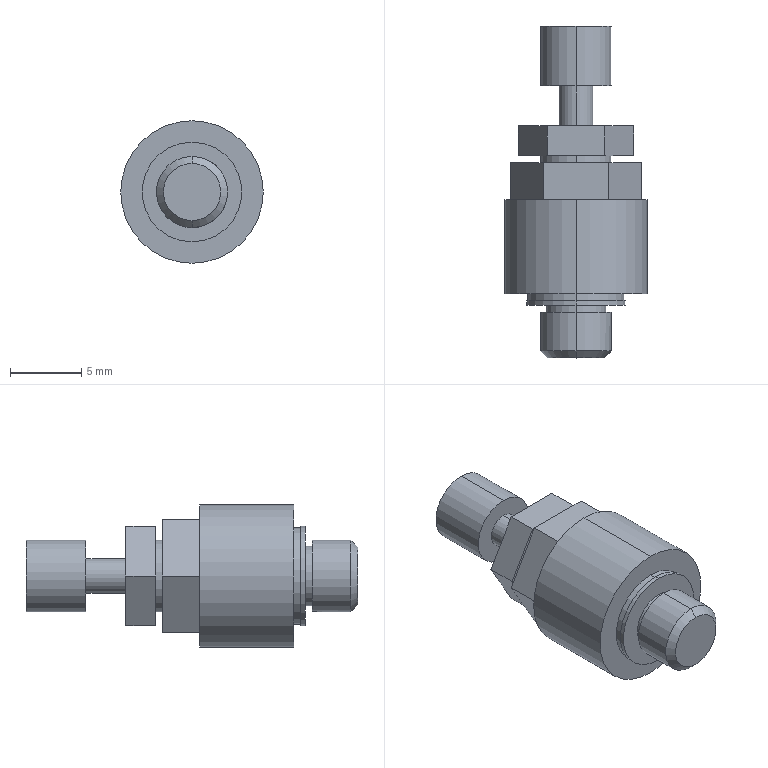Part | SolidWorks | features BaseBody 1 | 1 solid | 41 faces | box 10 x 23.3 x 10 mm | volume 954.231 mm3 | plane 23 | cylinder 16 | cone 2 | commonest cylinder face diameters 5 x6 2.4 x2 4.2 x2 6.8 x2 7 x2 10 x2
STEP:
#1=CARTESIAN_POINT('',(-2.309,6.6,4.));
#2=VERTEX_POINT('',#1);
#3=CARTESIAN_POINT('',(2.309,6.6,4.));
#4=VERTEX_POINT('',#3);
#5=CARTESIAN_POINT('',(0.,6.6,4.));
#6=DIRECTION('',(1.,0.,0.));
#7=VECTOR('',#6,1000.);
#8=LINE('',#5,#7);
#9=EDGE_CURVE('',#2,#4,#8,.T.);
#10=ORIENTED_EDGE('',*,*,#9,.F.);
#11=CARTESIAN_POINT('',(-4.619,6.6,0.));
#12=VERTEX_POINT('',#11);
#13=CARTESIAN_POINT('',(-4.619,6.6,0.));
#14=DIRECTION('',(0.5,0.,0.866));
#15=VECTOR('',#14,1000.);
#16=LINE('',#13,#15);
#17=EDGE_CURVE('',#12,#2,#16,.T.);
#18=ORIENTED_EDGE('',*,*,#17,.F.);
#19=CARTESIAN_POINT('',(-2.309,6.6,-4.));
#20=VERTEX_POINT('',#19);
#21=CARTESIAN_POINT('',(-2.309,6.6,-4.));
#22=DIRECTION('',(-0.5,0.,0.866));
#23=VECTOR('',#22,1000.);
#24=LINE('',#21,#23);
#25=EDGE_CURVE('',#20,#12,#24,.T.);
#26=ORIENTED_EDGE('',*,*,#25,.F.);
#27=CARTESIAN_POINT('',(2.309,6.6,-4.));
#28=VERTEX_POINT('',#27);
#29=CARTESIAN_POINT('',(2.309,6.6,-4.));
#30=DIRECTION('',(-1.,0.,0.));
#31=VECTOR('',#30,1000.);
#32=LINE('',#29,#31);
#33=EDGE_CURVE('',#28,#20,#32,.T.);
#34=ORIENTED_EDGE('',*,*,#33,.F.);
#35=CARTESIAN_POINT('',(4.619,6.6,0.));
#36=VERTEX_POINT('',#35);
#37=CARTESIAN_POINT('',(4.619,6.6,0.));
#38=DIRECTION('',(-0.5,0.,-0.866));
#39=VECTOR('',#38,1000.);
#40=LINE('',#37,#39);
#41=EDGE_CURVE('',#36,#28,#40,.T.);
#42=ORIENTED_EDGE('',*,*,#41,.F.);
#43=CARTESIAN_POINT('',(2.309,6.6,4.));
#44=DIRECTION('',(0.5,0.,-0.866));
#45=VECTOR('',#44,1000.);
#46=LINE('',#43,#45);
#47=EDGE_CURVE('',#4,#36,#46,.T.);
#48=ORIENTED_EDGE('',*,*,#47,.F.);
#49=EDGE_LOOP('',(#10,#18,#26,#34,#42,#48));
#50=FACE_BOUND('',#49,.T.);
#51=CARTESIAN_POINT('',(0.,6.6,5.));
#52=VERTEX_POINT('',#51);
#53=CARTESIAN_POINT('',(0.,6.6,-5.));
#54=VERTEX_POINT('',#53);
#55=CARTESIAN_POINT('',(0.,6.6,0.));
#56=DIRECTION('',(0.,1.,0.));
#57=DIRECTION('',(0.,0.,1.));
#58=AXIS2_PLACEMENT_3D('',#55,#56,#57);
#59=CIRCLE('',#58,5.);
#60=EDGE_CURVE('',#52,#54,#59,.T.);
#61=ORIENTED_EDGE('',*,*,#60,.T.);
#62=CARTESIAN_POINT('',(0.,6.6,0.));
#63=DIRECTION('',(0.,1.,0.));
#64=DIRECTION('',(0.,0.,1.));
#65=AXIS2_PLACEMENT_3D('',#62,#63,#64);
#66=CIRCLE('',#65,5.);
#67=EDGE_CURVE('',#54,#52,#66,.T.);
#68=ORIENTED_EDGE('',*,*,#67,.T.);
#69=EDGE_LOOP('',(#61,#68));
#70=FACE_OUTER_BOUND('',#69,.T.);
#71=CARTESIAN_POINT('',(0.,6.6,5.));
#72=DIRECTION('',(0.,-1.,0.));
#73=DIRECTION('',(0.,0.,-1.));
#74=AXIS2_PLACEMENT_3D('',#71,#72,#73);
#75=PLANE('',#74);
#76=ADVANCED_FACE('',(#50,#70),#75,.F.);
#77=CARTESIAN_POINT('',(0.,0.,-5.));
#78=VERTEX_POINT('',#77);
#79=CARTESIAN_POINT('',(0.,0.,-5.));
#80=DIRECTION('',(0.,1.,0.));
#81=VECTOR('',#80,1000.);
#82=LINE('',#79,#81);
#83=EDGE_CURVE('',#78,#54,#82,.T.);
#84=ORIENTED_EDGE('',*,*,#83,.F.);
#85=CARTESIAN_POINT('',(0.,0.,5.));
#86=VERTEX_POINT('',#85);
#87=CARTESIAN_POINT('',(0.,0.,0.));
#88=DIRECTION('',(0.,1.,0.));
#89=DIRECTION('',(0.,0.,1.));
#90=AXIS2_PLACEMENT_3D('',#87,#88,#89);
#91=CIRCLE('',#90,5.);
#92=EDGE_CURVE('',#78,#86,#91,.T.);
#93=ORIENTED_EDGE('',*,*,#92,.T.);
#94=CARTESIAN_POINT('',(0.,0.,5.));
#95=DIRECTION('',(0.,1.,0.));
#96=VECTOR('',#95,1000.);
#97=LINE('',#94,#96);
#98=EDGE_CURVE('',#86,#52,#97,.T.);
#99=ORIENTED_EDGE('',*,*,#98,.T.);
#100=ORIENTED_EDGE('',*,*,#67,.F.);
#101=EDGE_LOOP('',(#84,#93,#99,#100));
#102=FACE_OUTER_BOUND('',#101,.T.);
#103=CARTESIAN_POINT('',(0.,6.6,0.));
#104=DIRECTION('',(0.,1.,0.));
#105=DIRECTION('',(1.,0.,0.));
#106=AXIS2_PLACEMENT_3D('',#103,#104,#105);
#107=CYLINDRICAL_SURFACE('',#106,5.);
#108=ADVANCED_FACE('',(#102),#107,.T.);
#109=ORIENTED_EDGE('',*,*,#83,.T.);
#110=ORIENTED_EDGE('',*,*,#60,.F.);
#111=ORIENTED_EDGE('',*,*,#98,.F.);
#112=CARTESIAN_POINT('',(0.,0.,0.));
#113=DIRECTION('',(0.,1.,0.));
#114=DIRECTION('',(0.,0.,1.));
#115=AXIS2_PLACEMENT_3D('',#112,#113,#114);
#116=CIRCLE('',#115,5.);
#117=EDGE_CURVE('',#86,#78,#116,.T.);
#118=ORIENTED_EDGE('',*,*,#117,.T.);
#119=EDGE_LOOP('',(#109,#110,#111,#118));
#120=FACE_OUTER_BOUND('',#119,.T.);
#121=CARTESIAN_POINT('',(0.,6.6,0.));
#122=DIRECTION('',(0.,1.,0.));
#123=DIRECTION('',(-1.,0.,0.));
#124=AXIS2_PLACEMENT_3D('',#121,#122,#123);
#125=CYLINDRICAL_SURFACE('',#124,5.);
#126=ADVANCED_FACE('',(#120),#125,.T.);
#127=ORIENTED_EDGE('',*,*,#92,.F.);
#128=ORIENTED_EDGE('',*,*,#117,.F.);
#129=EDGE_LOOP('',(#127,#128));
#130=FACE_OUTER_BOUND('',#129,.T.);
#131=CARTESIAN_POINT('',(0.,0.,3.4));
#132=VERTEX_POINT('',#131);
#133=CARTESIAN_POINT('',(0.,0.,-3.4));
#134=VERTEX_POINT('',#133);
#135=CARTESIAN_POINT('',(0.,0.,0.));
#136=DIRECTION('',(0.,1.,0.));
#137=DIRECTION('',(0.,0.,1.));
#138=AXIS2_PLACEMENT_3D('',#135,#136,#137);
#139=CIRCLE('',#138,3.4);
#140=EDGE_CURVE('',#132,#134,#139,.T.);
#141=ORIENTED_EDGE('',*,*,#140,.T.);
#142=CARTESIAN_POINT('',(0.,0.,0.));
#143=DIRECTION('',(0.,1.,0.));
#144=DIRECTION('',(0.,0.,1.));
#145=AXIS2_PLACEMENT_3D('',#142,#143,#144);
#146=CIRCLE('',#145,3.4);
#147=EDGE_CURVE('',#134,#132,#146,.T.);
#148=ORIENTED_EDGE('',*,*,#147,.T.);
#149=EDGE_LOOP('',(#141,#148));
#150=FACE_BOUND('',#149,.T.);
#151=CARTESIAN_POINT('',(0.,0.,3.4));
#152=DIRECTION('',(0.,1.,0.));
#153=DIRECTION('',(0.,0.,1.));
#154=AXIS2_PLACEMENT_3D('',#151,#152,#153);
#155=PLANE('',#154);
#156=ADVANCED_FACE('',(#130,#150),#155,.F.);
#157=CARTESIAN_POINT('',(0.,-0.5,-3.4));
#158=VERTEX_POINT('',#157);
#159=CARTESIAN_POINT('',(0.,-0.5,-3.4));
#160=DIRECTION('',(0.,1.,0.));
#161=VECTOR('',#160,1000.);
#162=LINE('',#159,#161);
#163=EDGE_CURVE('',#158,#134,#162,.T.);
#164=ORIENTED_EDGE('',*,*,#163,.F.);
#165=CARTESIAN_POINT('',(0.,-0.5,3.4));
#166=VERTEX_POINT('',#165);
#167=CARTESIAN_POINT('',(0.,-0.5,0.));
#168=DIRECTION('',(0.,1.,0.));
#169=DIRECTION('',(0.,0.,1.));
#170=AXIS2_PLACEMENT_3D('',#167,#168,#169);
#171=CIRCLE('',#170,3.4);
#172=EDGE_CURVE('',#158,#166,#171,.T.);
#173=ORIENTED_EDGE('',*,*,#172,.T.);
#174=CARTESIAN_POINT('',(0.,-0.5,3.4));
#175=DIRECTION('',(0.,1.,0.));
#176=VECTOR('',#175,1000.);
#177=LINE('',#174,#176);
#178=EDGE_CURVE('',#166,#132,#177,.T.);
#179=ORIENTED_EDGE('',*,*,#178,.T.);
#180=ORIENTED_EDGE('',*,*,#147,.F.);
#181=EDGE_LOOP('',(#164,#173,#179,#180));
#182=FACE_OUTER_BOUND('',#181,.T.);
#183=CARTESIAN_POINT('',(0.,6.6,0.));
#184=DIRECTION('',(0.,1.,0.));
#185=DIRECTION('',(1.,0.,0.));
#186=AXIS2_PLACEMENT_3D('',#183,#184,#185);
#187=CYLINDRICAL_SURFACE('',#186,3.4);
#188=ADVANCED_FACE('',(#182),#187,.T.);
#189=ORIENTED_EDGE('',*,*,#163,.T.);
#190=ORIENTED_EDGE('',*,*,#140,.F.);
#191=ORIENTED_EDGE('',*,*,#178,.F.);
#192=CARTESIAN_POINT('',(0.,-0.5,0.));
#193=DIRECTION('',(0.,1.,0.));
#194=DIRECTION('',(0.,0.,1.));
#195=AXIS2_PLACEMENT_3D('',#192,#193,#194);
#196=CIRCLE('',#195,3.4);
#197=EDGE_CURVE('',#166,#158,#196,.T.);
#198=ORIENTED_EDGE('',*,*,#197,.T.);
#199=EDGE_LOOP('',(#189,#190,#191,#198));
#200=FACE_OUTER_BOUND('',#199,.T.);
#201=CARTESIAN_POINT('',(0.,6.6,0.));
#202=DIRECTION('',(0.,1.,0.));
#203=DIRECTION('',(-1.,0.,0.));
#204=AXIS2_PLACEMENT_3D('',#201,#202,#203);
#205=CYLINDRICAL_SURFACE('',#204,3.4);
#206=ADVANCED_FACE('',(#200),#205,.T.);
#207=ORIENTED_EDGE('',*,*,#172,.F.);
#208=ORIENTED_EDGE('',*,*,#197,.F.);
#209=EDGE_LOOP('',(#207,#208));
#210=FACE_BOUND('',#209,.T.);
#211=CARTESIAN_POINT('',(0.,-0.5,3.5));
#212=VERTEX_POINT('',#211);
#213=CARTESIAN_POINT('',(0.,-0.5,-3.5));
#214=VERTEX_POINT('',#213);
#215=CARTESIAN_POINT('',(0.,-0.5,0.));
#216=DIRECTION('',(0.,1.,0.));
#217=DIRECTION('',(0.,0.,1.));
#218=AXIS2_PLACEMENT_3D('',#215,#216,#217);
#219=CIRCLE('',#218,3.5);
#220=EDGE_CURVE('',#212,#214,#219,.T.);
#221=ORIENTED_EDGE('',*,*,#220,.T.);
#222=CARTESIAN_POINT('',(0.,-0.5,0.));
#223=DIRECTION('',(0.,1.,0.));
#224=DIRECTION('',(0.,0.,1.));
#225=AXIS2_PLACEMENT_3D('',#222,#223,#224);
#226=CIRCLE('',#225,3.5);
#227=EDGE_CURVE('',#214,#212,#226,.T.);
#228=ORIENTED_EDGE('',*,*,#227,.T.);
#229=EDGE_LOOP('',(#221,#228));
#230=FACE_OUTER_BOUND('',#229,.T.);
#231=CARTESIAN_POINT('',(0.,-0.5,3.5));
#232=DIRECTION('',(0.,-1.,0.));
#233=DIRECTION('',(0.,0.,-1.));
#234=AXIS2_PLACEMENT_3D('',#231,#232,#233);
#235=PLANE('',#234);
#236=ADVANCED_FACE('',(#210,#230),#235,.F.);
#237=CARTESIAN_POINT('',(0.,-0.8,-3.5));
#238=VERTEX_POINT('',#237);
#239=CARTESIAN_POINT('',(0.,-0.8,-3.5));
#240=DIRECTION('',(0.,1.,0.));
#241=VECTOR('',#240,1000.);
#242=LINE('',#239,#241);
#243=EDGE_CURVE('',#238,#214,#242,.T.);
#244=ORIENTED_EDGE('',*,*,#243,.F.);
#245=CARTESIAN_POINT('',(0.,-0.8,3.5));
#246=VERTEX_POINT('',#245);
#247=CARTESIAN_POINT('',(0.,-0.8,0.));
#248=DIRECTION('',(0.,1.,0.));
#249=DIRECTION('',(0.,0.,1.));
#250=AXIS2_PLACEMENT_3D('',#247,#248,#249);
#251=CIRCLE('',#250,3.5);
#252=EDGE_CURVE('',#238,#246,#251,.T.);
#253=ORIENTED_EDGE('',*,*,#252,.T.);
#254=CARTESIAN_POINT('',(0.,-0.8,3.5));
#255=DIRECTION('',(0.,1.,0.));
#256=VECTOR('',#255,1000.);
#257=LINE('',#254,#256);
#258=EDGE_CURVE('',#246,#212,#257,.T.);
#259=ORIENTED_EDGE('',*,*,#258,.T.);
#260=ORIENTED_EDGE('',*,*,#227,.F.);
#261=EDGE_LOOP('',(#244,#253,#259,#260));
#262=FACE_OUTER_BOUND('',#261,.T.);
#263=CARTESIAN_POINT('',(0.,6.6,0.));
#264=DIRECTION('',(0.,1.,0.));
#265=DIRECTION('',(1.,0.,0.));
#266=AXIS2_PLACEMENT_3D('',#263,#264,#265);
#267=CYLINDRICAL_SURFACE('',#266,3.5);
#268=ADVANCED_FACE('',(#262),#267,.T.);
#269=ORIENTED_EDGE('',*,*,#243,.T.);
#270=ORIENTED_EDGE('',*,*,#220,.F.);
#271=ORIENTED_EDGE('',*,*,#258,.F.);
#272=CARTESIAN_POINT('',(0.,-0.8,0.));
#273=DIRECTION('',(0.,1.,0.));
#274=DIRECTION('',(0.,0.,1.));
#275=AXIS2_PLACEMENT_3D('',#272,#273,#274);
#276=CIRCLE('',#275,3.5);
#277=EDGE_CURVE('',#246,#238,#276,.T.);
#278=ORIENTED_EDGE('',*,*,#277,.T.);
#279=EDGE_LOOP('',(#269,#270,#271,#278));
#280=FACE_OUTER_BOUND('',#279,.T.);
#281=CARTESIAN_POINT('',(0.,6.6,0.));
#282=DIRECTION('',(0.,1.,0.));
#283=DIRECTION('',(-1.,0.,0.));
#284=AXIS2_PLACEMENT_3D('',#281,#282,#283);
#285=CYLINDRICAL_SURFACE('',#284,3.5);
#286=ADVANCED_FACE('',(#280),#285,.T.);
#287=ORIENTED_EDGE('',*,*,#252,.F.);
#288=ORIENTED_EDGE('',*,*,#277,.F.);
#289=EDGE_LOOP('',(#287,#288));
#290=FACE_OUTER_BOUND('',#289,.T.);
#291=CARTESIAN_POINT('',(0.,-0.8,2.1));
#292=VERTEX_POINT('',#291);
#293=CARTESIAN_POINT('',(0.,-0.8,-2.1));
#294=VERTEX_POINT('',#293);
#295=CARTESIAN_POINT('',(0.,-0.8,0.));
#296=DIRECTION('',(0.,1.,0.));
#297=DIRECTION('',(0.,0.,1.));
#298=AXIS2_PLACEMENT_3D('',#295,#296,#297);
#299=CIRCLE('',#298,2.1);
#300=EDGE_CURVE('',#292,#294,#299,.T.);
#301=ORIENTED_EDGE('',*,*,#300,.T.);
#302=CARTESIAN_POINT('',(0.,-0.8,0.));
#303=DIRECTION('',(0.,1.,0.));
#304=DIRECTION('',(0.,0.,1.));
#305=AXIS2_PLACEMENT_3D('',#302,#303,#304);
#306=CIRCLE('',#305,2.1);
#307=EDGE_CURVE('',#294,#292,#306,.T.);
#308=ORIENTED_EDGE('',*,*,#307,.T.);
#309=EDGE_LOOP('',(#301,#308));
#310=FACE_BOUND('',#309,.T.);
#311=CARTESIAN_POINT('',(0.,-0.8,2.1));
#312=DIRECTION('',(0.,1.,0.));
#313=DIRECTION('',(0.,0.,1.));
#314=AXIS2_PLACEMENT_3D('',#311,#312,#313);
#315=PLANE('',#314);
#316=ADVANCED_FACE('',(#290,#310),#315,.F.);
#317=CARTESIAN_POINT('',(0.,-1.3,-2.1));
#318=VERTEX_POINT('',#317);
#319=CARTESIAN_POINT('',(0.,-1.3,-2.1));
#320=DIRECTION('',(0.,1.,0.));
#321=VECTOR('',#320,1000.);
#322=LINE('',#319,#321);
#323=EDGE_CURVE('',#318,#294,#322,.T.);
#324=ORIENTED_EDGE('',*,*,#323,.F.);
#325=CARTESIAN_POINT('',(0.,-1.3,2.1));
#326=VERTEX_POINT('',#325);
#327=CARTESIAN_POINT('',(0.,-1.3,0.));
#328=DIRECTION('',(0.,1.,0.));
#329=DIRECTION('',(0.,0.,1.));
#330=AXIS2_PLACEMENT_3D('',#327,#328,#329);
#331=CIRCLE('',#330,2.1);
#332=EDGE_CURVE('',#318,#326,#331,.T.);
#333=ORIENTED_EDGE('',*,*,#332,.T.);
#334=CARTESIAN_POINT('',(0.,-1.3,2.1));
#335=DIRECTION('',(0.,1.,0.));
#336=VECTOR('',#335,1000.);
#337=LINE('',#334,#336);
#338=EDGE_CURVE('',#326,#292,#337,.T.);
#339=ORIENTED_EDGE('',*,*,#338,.T.);
#340=ORIENTED_EDGE('',*,*,#307,.F.);
#341=EDGE_LOOP('',(#324,#333,#339,#340));
#342=FACE_OUTER_BOUND('',#341,.T.);
#343=CARTESIAN_POINT('',(0.,6.6,0.));
#344=DIRECTION('',(0.,1.,0.));
#345=DIRECTION('',(1.,0.,0.));
#346=AXIS2_PLACEMENT_3D('',#343,#344,#345);
#347=CYLINDRICAL_SURFACE('',#346,2.1);
#348=ADVANCED_FACE('',(#342),#347,.T.);
#349=ORIENTED_EDGE('',*,*,#323,.T.);
#350=ORIENTED_EDGE('',*,*,#300,.F.);
#351=ORIENTED_EDGE('',*,*,#338,.F.);
#352=CARTESIAN_POINT('',(0.,-1.3,0.));
#353=DIRECTION('',(0.,1.,0.));
#354=DIRECTION('',(0.,0.,1.));
#355=AXIS2_PLACEMENT_3D('',#352,#353,#354);
#356=CIRCLE('',#355,2.1);
#357=EDGE_CURVE('',#326,#318,#356,.T.);
#358=ORIENTED_EDGE('',*,*,#357,.T.);
#359=EDGE_LOOP('',(#349,#350,#351,#358));
#360=FACE_OUTER_BOUND('',#359,.T.);
#361=CARTESIAN_POINT('',(0.,6.6,0.));
#362=DIRECTION('',(0.,1.,0.));
#363=DIRECTION('',(-1.,0.,0.));
#364=AXIS2_PLACEMENT_3D('',#361,#362,#363);
#365=CYLINDRICAL_SURFACE('',#364,2.1);
#366=ADVANCED_FACE('',(#360),#365,.T.);
#367=ORIENTED_EDGE('',*,*,#332,.F.);
#368=ORIENTED_EDGE('',*,*,#357,.F.);
#369=EDGE_LOOP('',(#367,#368));
#370=FACE_BOUND('',#369,.T.);
#371=CARTESIAN_POINT('',(0.,-1.3,2.5));
#372=VERTEX_POINT('',#371);
#373=CARTESIAN_POINT('',(-0.7725,-1.3,-2.378));
#374=VERTEX_POINT('',#373);
#375=CARTESIAN_POINT('',(0.,-1.3,0.));
#376=DIRECTION('',(0.,1.,0.));
#377=DIRECTION('',(0.,0.,1.));
#378=AXIS2_PLACEMENT_3D('',#375,#376,#377);
#379=CIRCLE('',#378,2.5);
#380=EDGE_CURVE('',#372,#374,#379,.T.);
#381=ORIENTED_EDGE('',*,*,#380,.T.);
#382=CARTESIAN_POINT('',(0.,-1.3,0.));
#383=DIRECTION('',(0.,1.,0.));
#384=DIRECTION('',(0.,0.,1.));
#385=AXIS2_PLACEMENT_3D('',#382,#383,#384);
#386=CIRCLE('',#385,2.5);
#387=EDGE_CURVE('',#374,#372,#386,.T.);
#388=ORIENTED_EDGE('',*,*,#387,.T.);
#389=EDGE_LOOP('',(#381,#388));
#390=FACE_OUTER_BOUND('',#389,.T.);
#391=CARTESIAN_POINT('',(0.,-1.3,2.5));
#392=DIRECTION('',(0.,-1.,0.));
#393=DIRECTION('',(0.,0.,-1.));
#394=AXIS2_PLACEMENT_3D('',#391,#392,#393);
#395=PLANE('',#394);
#396=ADVANCED_FACE('',(#370,#390),#395,.F.);
#397=CARTESIAN_POINT('',(-0.7725,-4.01,-2.378));
#398=VERTEX_POINT('',#397);
#399=CARTESIAN_POINT('',(-0.7725,-4.01,-2.378));
#400=DIRECTION('',(0.,1.,0.));
#401=VECTOR('',#400,1000.);
#402=LINE('',#399,#401);
#403=EDGE_CURVE('',#398,#374,#402,.T.);
#404=ORIENTED_EDGE('',*,*,#403,.F.);
#405=CARTESIAN_POINT('',(0.,-4.01,2.5));
#406=VERTEX_POINT('',#405);
#407=CARTESIAN_POINT('',(0.,-4.01,0.));
#408=DIRECTION('',(0.,1.,0.));
#409=DIRECTION('',(0.,0.,1.));
#410=AXIS2_PLACEMENT_3D('',#407,#408,#409);
#411=CIRCLE('',#410,2.5);
#412=EDGE_CURVE('',#398,#406,#411,.T.);
#413=ORIENTED_EDGE('',*,*,#412,.T.);
#414=CARTESIAN_POINT('',(0.,-4.01,2.5));
#415=DIRECTION('',(0.,1.,0.));
#416=VECTOR('',#415,1000.);
#417=LINE('',#414,#416);
#418=EDGE_CURVE('',#406,#372,#417,.T.);
#419=ORIENTED_EDGE('',*,*,#418,.T.);
#420=ORIENTED_EDGE('',*,*,#387,.F.);
#421=EDGE_LOOP('',(#404,#413,#419,#420));
#422=FACE_OUTER_BOUND('',#421,.T.);
#423=CARTESIAN_POINT('',(0.,6.6,0.));
#424=DIRECTION('',(0.,1.,0.));
#425=DIRECTION('',(0.9877,0.,-0.1564));
#426=AXIS2_PLACEMENT_3D('',#423,#424,#425);
#427=CYLINDRICAL_SURFACE('',#426,2.5);
#428=ADVANCED_FACE('',(#422),#427,.T.);
#429=ORIENTED_EDGE('',*,*,#403,.T.);
#430=ORIENTED_EDGE('',*,*,#380,.F.);
#431=ORIENTED_EDGE('',*,*,#418,.F.);
#432=CARTESIAN_POINT('',(0.,-4.01,-2.5));
#433=VERTEX_POINT('',#432);
#434=CARTESIAN_POINT('',(0.,-4.01,0.));
#435=DIRECTION('',(0.,1.,0.));
#436=DIRECTION('',(0.,0.,1.));
#437=AXIS2_PLACEMENT_3D('',#434,#435,#436);
#438=CIRCLE('',#437,2.5);
#439=EDGE_CURVE('',#406,#433,#438,.T.);
#440=ORIENTED_EDGE('',*,*,#439,.T.);
#441=CARTESIAN_POINT('',(0.,-4.01,0.));
#442=DIRECTION('',(0.,1.,0.));
#443=DIRECTION('',(0.,0.,1.));
#444=AXIS2_PLACEMENT_3D('',#441,#442,#443);
#445=CIRCLE('',#444,2.5);
#446=EDGE_CURVE('',#433,#398,#445,.T.);
#447=ORIENTED_EDGE('',*,*,#446,.T.);
#448=EDGE_LOOP('',(#429,#430,#431,#440,#447));
#449=FACE_OUTER_BOUND('',#448,.T.);
#450=CARTESIAN_POINT('',(0.,6.6,0.));
#451=DIRECTION('',(0.,1.,0.));
#452=DIRECTION('',(-0.9877,0.,0.1564));
#453=AXIS2_PLACEMENT_3D('',#450,#451,#452);
#454=CYLINDRICAL_SURFACE('',#453,2.5);
#455=ADVANCED_FACE('',(#449),#454,.T.);
#456=CARTESIAN_POINT('',(0.,-4.5,-2.01));
#457=VERTEX_POINT('',#456);
#458=CARTESIAN_POINT('',(0.,-4.5,-2.01));
#459=DIRECTION('',(0.,0.7071,-0.7071));
#460=VECTOR('',#459,1000.);
#461=LINE('',#458,#460);
#462=EDGE_CURVE('',#457,#433,#461,.T.);
#463=ORIENTED_EDGE('',*,*,#462,.F.);
#464=CARTESIAN_POINT('',(0.,-4.5,2.01));
#465=VERTEX_POINT('',#464);
#466=CARTESIAN_POINT('',(0.,-4.5,0.));
#467=DIRECTION('',(0.,1.,0.));
#468=DIRECTION('',(0.,0.,1.));
#469=AXIS2_PLACEMENT_3D('',#466,#467,#468);
#470=CIRCLE('',#469,2.01);
#471=EDGE_CURVE('',#457,#465,#470,.T.);
#472=ORIENTED_EDGE('',*,*,#471,.T.);
#473=CARTESIAN_POINT('',(0.,-4.5,2.01));
#474=DIRECTION('',(0.,0.7071,0.7071));
#475=VECTOR('',#474,1000.);
#476=LINE('',#473,#475);
#477=EDGE_CURVE('',#465,#406,#476,.T.);
#478=ORIENTED_EDGE('',*,*,#477,.T.);
#479=ORIENTED_EDGE('',*,*,#412,.F.);
#480=ORIENTED_EDGE('',*,*,#446,.F.);
#481=EDGE_LOOP('',(#463,#472,#478,#479,#480));
#482=FACE_OUTER_BOUND('',#481,.T.);
#483=CARTESIAN_POINT('',(0.,-4.5,0.));
#484=DIRECTION('',(0.,1.,0.));
#485=DIRECTION('',(1.,0.,0.));
#486=AXIS2_PLACEMENT_3D('',#483,#484,#485);
#487=CONICAL_SURFACE('',#486,2.01,0.7854);
#488=ADVANCED_FACE('',(#482),#487,.T.);
#489=ORIENTED_EDGE('',*,*,#462,.T.);
#490=ORIENTED_EDGE('',*,*,#439,.F.);
#491=ORIENTED_EDGE('',*,*,#477,.F.);
#492=CARTESIAN_POINT('',(0.,-4.5,0.));
#493=DIRECTION('',(0.,1.,0.));
#494=DIRECTION('',(0.,0.,1.));
#495=AXIS2_PLACEMENT_3D('',#492,#493,#494);
#496=CIRCLE('',#495,2.01);
#497=EDGE_CURVE('',#465,#457,#496,.T.);
#498=ORIENTED_EDGE('',*,*,#497,.T.);
#499=EDGE_LOOP('',(#489,#490,#491,#498));
#500=FACE_OUTER_BOUND('',#499,.T.);
#501=CARTESIAN_POINT('',(0.,-4.5,0.));
#502=DIRECTION('',(0.,1.,0.));
#503=DIRECTION('',(-1.,0.,0.));
#504=AXIS2_PLACEMENT_3D('',#501,#502,#503);
#505=CONICAL_SURFACE('',#504,2.01,0.7854);
#506=ADVANCED_FACE('',(#500),#505,.T.);
#507=ORIENTED_EDGE('',*,*,#471,.F.);
#508=ORIENTED_EDGE('',*,*,#497,.F.);
#509=EDGE_LOOP('',(#507,#508));
#510=FACE_OUTER_BOUND('',#509,.T.);
#511=CARTESIAN_POINT('',(0.,-4.5,0.));
#512=DIRECTION('',(0.,1.,0.));
#513=DIRECTION('',(0.,0.,1.));
#514=AXIS2_PLACEMENT_3D('',#511,#512,#513);
#515=PLANE('',#514);
#516=ADVANCED_FACE('',(#510),#515,.F.);
#517=ORIENTED_EDGE('',*,*,#47,.T.);
#518=CARTESIAN_POINT('',(4.619,9.2,0.));
#519=VERTEX_POINT('',#518);
#520=CARTESIAN_POINT('',(4.619,9.2,0.));
#521=DIRECTION('',(0.,-1.,0.));
#522=VECTOR('',#521,1000.);
#523=LINE('',#520,#522);
#524=EDGE_CURVE('',#519,#36,#523,.T.);
#525=ORIENTED_EDGE('',*,*,#524,.F.);
#526=CARTESIAN_POINT('',(2.309,9.2,4.));
#527=VERTEX_POINT('',#526);
#528=CARTESIAN_POINT('',(2.309,9.2,4.));
#529=DIRECTION('',(0.5,0.,-0.866));
#530=VECTOR('',#529,1000.);
#531=LINE('',#528,#530);
#532=EDGE_CURVE('',#527,#519,#531,.T.);
#533=ORIENTED_EDGE('',*,*,#532,.F.);
#534=CARTESIAN_POINT('',(2.309,9.2,4.));
#535=DIRECTION('',(0.,-1.,0.));
#536=VECTOR('',#535,1000.);
#537=LINE('',#534,#536);
#538=EDGE_CURVE('',#527,#4,#537,.T.);
#539=ORIENTED_EDGE('',*,*,#538,.T.);
#540=EDGE_LOOP('',(#517,#525,#533,#539));
#541=FACE_OUTER_BOUND('',#540,.T.);
#542=CARTESIAN_POINT('',(2.309,9.2,4.));
#543=DIRECTION('',(-0.866,0.,-0.5));
#544=DIRECTION('',(-0.5,0.,0.866));
#545=AXIS2_PLACEMENT_3D('',#542,#543,#544);
#546=PLANE('',#545);
#547=ADVANCED_FACE('',(#541),#546,.F.);
#548=CARTESIAN_POINT('',(-2.309,9.2,4.));
#549=VERTEX_POINT('',#548);
#550=CARTESIAN_POINT('',(-2.309,9.2,4.));
#551=DIRECTION('',(0.,-1.,0.));
#552=VECTOR('',#551,1000.);
#553=LINE('',#550,#552);
#554=EDGE_CURVE('',#549,#2,#553,.T.);
#555=ORIENTED_EDGE('',*,*,#554,.T.);
#556=ORIENTED_EDGE('',*,*,#9,.T.);
#557=ORIENTED_EDGE('',*,*,#538,.F.);
#558=CARTESIAN_POINT('',(-2.309,9.2,4.));
#559=DIRECTION('',(1.,0.,0.));
#560=VECTOR('',#559,1000.);
#561=LINE('',#558,#560);
#562=EDGE_CURVE('',#549,#527,#561,.T.);
#563=ORIENTED_EDGE('',*,*,#562,.F.);
#564=EDGE_LOOP('',(#555,#556,#557,#563));
#565=FACE_OUTER_BOUND('',#564,.T.);
#566=CARTESIAN_POINT('',(-2.309,9.2,4.));
#567=DIRECTION('',(0.,0.,-1.));
#568=DIRECTION('',(-1.,0.,0.));
#569=AXIS2_PLACEMENT_3D('',#566,#567,#568);
#570=PLANE('',#569);
#571=ADVANCED_FACE('',(#565),#570,.F.);
#572=CARTESIAN_POINT('',(0.,9.2,-2.5));
#573=VERTEX_POINT('',#572);
#574=CARTESIAN_POINT('',(0.,9.2,2.5));
#575=VERTEX_POINT('',#574);
#576=CARTESIAN_POINT('',(0.,9.2,0.));
#577=DIRECTION('',(0.,1.,0.));
#578=DIRECTION('',(0.,0.,1.));
#579=AXIS2_PLACEMENT_3D('',#576,#577,#578);
#580=CIRCLE('',#579,2.5);
#581=EDGE_CURVE('',#573,#575,#580,.T.);
#582=ORIENTED_EDGE('',*,*,#581,.F.);
#583=CARTESIAN_POINT('',(0.,9.2,0.));
#584=DIRECTION('',(0.,1.,0.));
#585=DIRECTION('',(0.,0.,1.));
#586=AXIS2_PLACEMENT_3D('',#583,#584,#585);
#587=CIRCLE('',#586,2.5);
#588=EDGE_CURVE('',#575,#573,#587,.T.);
#589=ORIENTED_EDGE('',*,*,#588,.F.);
#590=EDGE_LOOP('',(#582,#589));
#591=FACE_BOUND('',#590,.T.);
#592=CARTESIAN_POINT('',(2.309,9.2,-4.));
#593=VERTEX_POINT('',#592);
#594=CARTESIAN_POINT('',(-2.309,9.2,-4.));
#595=VERTEX_POINT('',#594);
#596=CARTESIAN_POINT('',(2.309,9.2,-4.));
#597=DIRECTION('',(-1.,0.,0.));
#598=VECTOR('',#597,1000.);
#599=LINE('',#596,#598);
#600=EDGE_CURVE('',#593,#595,#599,.T.);
#601=ORIENTED_EDGE('',*,*,#600,.T.);
#602=CARTESIAN_POINT('',(-4.619,9.2,0.));
#603=VERTEX_POINT('',#602);
#604=CARTESIAN_POINT('',(-2.309,9.2,-4.));
#605=DIRECTION('',(-0.5,0.,0.866));
#606=VECTOR('',#605,1000.);
#607=LINE('',#604,#606);
#608=EDGE_CURVE('',#595,#603,#607,.T.);
#609=ORIENTED_EDGE('',*,*,#608,.T.);
#610=CARTESIAN_POINT('',(-4.619,9.2,0.));
#611=DIRECTION('',(0.5,0.,0.866));
#612=VECTOR('',#611,1000.);
#613=LINE('',#610,#612);
#614=EDGE_CURVE('',#603,#549,#613,.T.);
#615=ORIENTED_EDGE('',*,*,#614,.T.);
#616=ORIENTED_EDGE('',*,*,#562,.T.);
#617=ORIENTED_EDGE('',*,*,#532,.T.);
#618=CARTESIAN_POINT('',(4.619,9.2,0.));
#619=DIRECTION('',(-0.5,0.,-0.866));
#620=VECTOR('',#619,1000.);
#621=LINE('',#618,#620);
#622=EDGE_CURVE('',#519,#593,#621,.T.);
#623=ORIENTED_EDGE('',*,*,#622,.T.);
#624=EDGE_LOOP('',(#601,#609,#615,#616,#617,#623));
#625=FACE_OUTER_BOUND('',#624,.T.);
#626=CARTESIAN_POINT('',(0.,9.2,0.));
#627=DIRECTION('',(0.,1.,0.));
#628=DIRECTION('',(0.,0.,1.));
#629=AXIS2_PLACEMENT_3D('',#626,#627,#628);
#630=PLANE('',#629);
#631=ADVANCED_FACE('',(#591,#625),#630,.T.);
#632=ORIENTED_EDGE('',*,*,#41,.T.);
#633=CARTESIAN_POINT('',(2.309,9.2,-4.));
#634=DIRECTION('',(0.,-1.,0.));
#635=VECTOR('',#634,1000.);
#636=LINE('',#633,#635);
#637=EDGE_CURVE('',#593,#28,#636,.T.);
#638=ORIENTED_EDGE('',*,*,#637,.F.);
#639=ORIENTED_EDGE('',*,*,#622,.F.);
#640=ORIENTED_EDGE('',*,*,#524,.T.);
#641=EDGE_LOOP('',(#632,#638,#639,#640));
#642=FACE_OUTER_BOUND('',#641,.T.);
#643=CARTESIAN_POINT('',(4.619,9.2,0.));
#644=DIRECTION('',(-0.866,0.,0.5));
#645=DIRECTION('',(0.5,0.,0.866));
#646=AXIS2_PLACEMENT_3D('',#643,#644,#645);
#647=PLANE('',#646);
#648=ADVANCED_FACE('',(#642),#647,.F.);
#649=ORIENTED_EDGE('',*,*,#33,.T.);
#650=CARTESIAN_POINT('',(-2.309,9.2,-4.));
#651=DIRECTION('',(0.,-1.,0.));
#652=VECTOR('',#651,1000.);
#653=LINE('',#650,#652);
#654=EDGE_CURVE('',#595,#20,#653,.T.);
#655=ORIENTED_EDGE('',*,*,#654,.F.);
#656=ORIENTED_EDGE('',*,*,#600,.F.);
#657=ORIENTED_EDGE('',*,*,#637,.T.);
#658=EDGE_LOOP('',(#649,#655,#656,#657));
#659=FACE_OUTER_BOUND('',#658,.T.);
#660=CARTESIAN_POINT('',(2.309,9.2,-4.));
#661=DIRECTION('',(0.,0.,1.));
#662=DIRECTION('',(1.,0.,0.));
#663=AXIS2_PLACEMENT_3D('',#660,#661,#662);
#664=PLANE('',#663);
#665=ADVANCED_FACE('',(#659),#664,.F.);
#666=ORIENTED_EDGE('',*,*,#25,.T.);
#667=CARTESIAN_POINT('',(-4.619,9.2,0.));
#668=DIRECTION('',(0.,-1.,0.));
#669=VECTOR('',#668,1000.);
#670=LINE('',#667,#669);
#671=EDGE_CURVE('',#603,#12,#670,.T.);
#672=ORIENTED_EDGE('',*,*,#671,.F.);
#673=ORIENTED_EDGE('',*,*,#608,.F.);
#674=ORIENTED_EDGE('',*,*,#654,.T.);
#675=EDGE_LOOP('',(#666,#672,#673,#674));
#676=FACE_OUTER_BOUND('',#675,.T.);
#677=CARTESIAN_POINT('',(-2.309,9.2,-4.));
#678=DIRECTION('',(0.866,0.,0.5));
#679=DIRECTION('',(0.5,0.,-0.866));
#680=AXIS2_PLACEMENT_3D('',#677,#678,#679);
#681=PLANE('',#680);
#682=ADVANCED_FACE('',(#676),#681,.F.);
#683=ORIENTED_EDGE('',*,*,#17,.T.);
#684=ORIENTED_EDGE('',*,*,#554,.F.);
#685=ORIENTED_EDGE('',*,*,#614,.F.);
#686=ORIENTED_EDGE('',*,*,#671,.T.);
#687=EDGE_LOOP('',(#683,#684,#685,#686));
#688=FACE_OUTER_BOUND('',#687,.T.);
#689=CARTESIAN_POINT('',(-4.619,9.2,0.));
#690=DIRECTION('',(0.866,0.,-0.5));
#691=DIRECTION('',(-0.5,0.,-0.866));
#692=AXIS2_PLACEMENT_3D('',#689,#690,#691);
#693=PLANE('',#692);
#694=ADVANCED_FACE('',(#688),#693,.F.);
#695=CARTESIAN_POINT('',(0.,9.7,-2.5));
#696=VERTEX_POINT('',#695);
#697=CARTESIAN_POINT('',(0.,9.2,-2.5));
#698=DIRECTION('',(0.,1.,0.));
#699=VECTOR('',#698,1000.);
#700=LINE('',#697,#699);
#701=EDGE_CURVE('',#573,#696,#700,.T.);
#702=ORIENTED_EDGE('',*,*,#701,.T.);
#703=CARTESIAN_POINT('',(0.,9.7,2.5));
#704=VERTEX_POINT('',#703);
#705=CARTESIAN_POINT('',(0.,9.7,0.));
#706=DIRECTION('',(0.,1.,0.));
#707=DIRECTION('',(0.,0.,1.));
#708=AXIS2_PLACEMENT_3D('',#705,#706,#707);
#709=CIRCLE('',#708,2.5);
#710=EDGE_CURVE('',#704,#696,#709,.T.);
#711=ORIENTED_EDGE('',*,*,#710,.F.);
#712=CARTESIAN_POINT('',(0.,9.2,2.5));
#713=DIRECTION('',(0.,1.,0.));
#714=VECTOR('',#713,1000.);
#715=LINE('',#712,#714);
#716=EDGE_CURVE('',#575,#704,#715,.T.);
#717=ORIENTED_EDGE('',*,*,#716,.F.);
#718=ORIENTED_EDGE('',*,*,#588,.T.);
#719=EDGE_LOOP('',(#702,#711,#717,#718));
#720=FACE_OUTER_BOUND('',#719,.T.);
#721=CARTESIAN_POINT('',(0.,18.8,0.));
#722=DIRECTION('',(0.,1.,0.));
#723=DIRECTION('',(-1.,0.,0.));
#724=AXIS2_PLACEMENT_3D('',#721,#722,#723);
#725=CYLINDRICAL_SURFACE('',#724,2.5);
#726=ADVANCED_FACE('',(#720),#725,.T.);
#727=ORIENTED_EDGE('',*,*,#701,.F.);
#728=ORIENTED_EDGE('',*,*,#581,.T.);
#729=ORIENTED_EDGE('',*,*,#716,.T.);
#730=CARTESIAN_POINT('',(0.,9.7,0.));
#731=DIRECTION('',(0.,1.,0.));
#732=DIRECTION('',(0.,0.,1.));
#733=AXIS2_PLACEMENT_3D('',#730,#731,#732);
#734=CIRCLE('',#733,2.5);
#735=EDGE_CURVE('',#696,#704,#734,.T.);
#736=ORIENTED_EDGE('',*,*,#735,.F.);
#737=EDGE_LOOP('',(#727,#728,#729,#736));
#738=FACE_OUTER_BOUND('',#737,.T.);
#739=CARTESIAN_POINT('',(0.,18.8,0.));
#740=DIRECTION('',(0.,1.,0.));
#741=DIRECTION('',(1.,0.,0.));
#742=AXIS2_PLACEMENT_3D('',#739,#740,#741);
#743=CYLINDRICAL_SURFACE('',#742,2.5);
#744=ADVANCED_FACE('',(#738),#743,.T.);
#745=CARTESIAN_POINT('',(2.021,9.7,3.5));
#746=VERTEX_POINT('',#745);
#747=CARTESIAN_POINT('',(-2.021,9.7,3.5));
#748=VERTEX_POINT('',#747);
#749=CARTESIAN_POINT('',(2.021,9.7,3.5));
#750=DIRECTION('',(-1.,0.,0.));
#751=VECTOR('',#750,1000.);
#752=LINE('',#749,#751);
#753=EDGE_CURVE('',#746,#748,#752,.T.);
#754=ORIENTED_EDGE('',*,*,#753,.T.);
#755=CARTESIAN_POINT('',(-4.041,9.7,0.));
#756=VERTEX_POINT('',#755);
#757=CARTESIAN_POINT('',(-2.021,9.7,3.5));
#758=DIRECTION('',(-0.5,0.,-0.866));
#759=VECTOR('',#758,1000.);
#760=LINE('',#757,#759);
#761=EDGE_CURVE('',#748,#756,#760,.T.);
#762=ORIENTED_EDGE('',*,*,#761,.T.);
#763=CARTESIAN_POINT('',(-2.021,9.7,-3.5));
#764=VERTEX_POINT('',#763);
#765=CARTESIAN_POINT('',(-4.041,9.7,0.));
#766=DIRECTION('',(0.5,0.,-0.866));
#767=VECTOR('',#766,1000.);
#768=LINE('',#765,#767);
#769=EDGE_CURVE('',#756,#764,#768,.T.);
#770=ORIENTED_EDGE('',*,*,#769,.T.);
#771=CARTESIAN_POINT('',(2.021,9.7,-3.5));
#772=VERTEX_POINT('',#771);
#773=CARTESIAN_POINT('',(-2.021,9.7,-3.5));
#774=DIRECTION('',(1.,0.,0.));
#775=VECTOR('',#774,1000.);
#776=LINE('',#773,#775);
#777=EDGE_CURVE('',#764,#772,#776,.T.);
#778=ORIENTED_EDGE('',*,*,#777,.T.);
#779=CARTESIAN_POINT('',(4.041,9.7,0.));
#780=VERTEX_POINT('',#779);
#781=CARTESIAN_POINT('',(2.021,9.7,-3.5));
#782=DIRECTION('',(0.5,0.,0.866));
#783=VECTOR('',#782,1000.);
#784=LINE('',#781,#783);
#785=EDGE_CURVE('',#772,#780,#784,.T.);
#786=ORIENTED_EDGE('',*,*,#785,.T.);
#787=CARTESIAN_POINT('',(4.041,9.7,0.));
#788=DIRECTION('',(-0.5,0.,0.866));
#789=VECTOR('',#788,1000.);
#790=LINE('',#787,#789);
#791=EDGE_CURVE('',#780,#746,#790,.T.);
#792=ORIENTED_EDGE('',*,*,#791,.T.);
#793=EDGE_LOOP('',(#754,#762,#770,#778,#786,#792));
#794=FACE_OUTER_BOUND('',#793,.T.);
#795=ORIENTED_EDGE('',*,*,#710,.T.);
#796=ORIENTED_EDGE('',*,*,#735,.T.);
#797=EDGE_LOOP('',(#795,#796));
#798=FACE_BOUND('',#797,.T.);
#799=CARTESIAN_POINT('',(0.,9.7,2.5));
#800=DIRECTION('',(0.,1.,0.));
#801=DIRECTION('',(0.,0.,1.));
#802=AXIS2_PLACEMENT_3D('',#799,#800,#801);
#803=PLANE('',#802);
#804=ADVANCED_FACE('',(#794,#798),#803,.F.);
#805=CARTESIAN_POINT('',(4.041,11.8,0.));
#806=VERTEX_POINT('',#805);
#807=CARTESIAN_POINT('',(2.021,11.8,3.5));
#808=VERTEX_POINT('',#807);
#809=CARTESIAN_POINT('',(4.041,11.8,0.));
#810=DIRECTION('',(-0.5,0.,0.866));
#811=VECTOR('',#810,1000.);
#812=LINE('',#809,#811);
#813=EDGE_CURVE('',#806,#808,#812,.T.);
#814=ORIENTED_EDGE('',*,*,#813,.T.);
#815=CARTESIAN_POINT('',(2.021,11.8,3.5));
#816=DIRECTION('',(0.,-1.,0.));
#817=VECTOR('',#816,1000.);
#818=LINE('',#815,#817);
#819=EDGE_CURVE('',#808,#746,#818,.T.);
#820=ORIENTED_EDGE('',*,*,#819,.T.);
#821=ORIENTED_EDGE('',*,*,#791,.F.);
#822=CARTESIAN_POINT('',(4.041,11.8,0.));
#823=DIRECTION('',(0.,-1.,0.));
#824=VECTOR('',#823,1000.);
#825=LINE('',#822,#824);
#826=EDGE_CURVE('',#806,#780,#825,.T.);
#827=ORIENTED_EDGE('',*,*,#826,.F.);
#828=EDGE_LOOP('',(#814,#820,#821,#827));
#829=FACE_OUTER_BOUND('',#828,.T.);
#830=CARTESIAN_POINT('',(4.041,11.8,0.));
#831=DIRECTION('',(0.866,0.,0.5));
#832=DIRECTION('',(0.5,0.,-0.866));
#833=AXIS2_PLACEMENT_3D('',#830,#831,#832);
#834=PLANE('',#833);
#835=ADVANCED_FACE('',(#829),#834,.T.);
#836=CARTESIAN_POINT('',(2.021,11.8,-3.5));
#837=VERTEX_POINT('',#836);
#838=CARTESIAN_POINT('',(2.021,11.8,-3.5));
#839=DIRECTION('',(0.5,0.,0.866));
#840=VECTOR('',#839,1000.);
#841=LINE('',#838,#840);
#842=EDGE_CURVE('',#837,#806,#841,.T.);
#843=ORIENTED_EDGE('',*,*,#842,.T.);
#844=ORIENTED_EDGE('',*,*,#826,.T.);
#845=ORIENTED_EDGE('',*,*,#785,.F.);
#846=CARTESIAN_POINT('',(2.021,11.8,-3.5));
#847=DIRECTION('',(0.,-1.,0.));
#848=VECTOR('',#847,1000.);
#849=LINE('',#846,#848);
#850=EDGE_CURVE('',#837,#772,#849,.T.);
#851=ORIENTED_EDGE('',*,*,#850,.F.);
#852=EDGE_LOOP('',(#843,#844,#845,#851));
#853=FACE_OUTER_BOUND('',#852,.T.);
#854=CARTESIAN_POINT('',(2.021,11.8,-3.5));
#855=DIRECTION('',(0.866,0.,-0.5));
#856=DIRECTION('',(-0.5,0.,-0.866));
#857=AXIS2_PLACEMENT_3D('',#854,#855,#856);
#858=PLANE('',#857);
#859=ADVANCED_FACE('',(#853),#858,.T.);
#860=CARTESIAN_POINT('',(-2.021,11.8,-3.5));
#861=VERTEX_POINT('',#860);
#862=CARTESIAN_POINT('',(-2.021,11.8,-3.5));
#863=DIRECTION('',(1.,0.,0.));
#864=VECTOR('',#863,1000.);
#865=LINE('',#862,#864);
#866=EDGE_CURVE('',#861,#837,#865,.T.);
#867=ORIENTED_EDGE('',*,*,#866,.T.);
#868=ORIENTED_EDGE('',*,*,#850,.T.);
#869=ORIENTED_EDGE('',*,*,#777,.F.);
#870=CARTESIAN_POINT('',(-2.021,11.8,-3.5));
#871=DIRECTION('',(0.,-1.,0.));
#872=VECTOR('',#871,1000.);
#873=LINE('',#870,#872);
#874=EDGE_CURVE('',#861,#764,#873,.T.);
#875=ORIENTED_EDGE('',*,*,#874,.F.);
#876=EDGE_LOOP('',(#867,#868,#869,#875));
#877=FACE_OUTER_BOUND('',#876,.T.);
#878=CARTESIAN_POINT('',(-2.021,11.8,-3.5));
#879=DIRECTION('',(0.,0.,-1.));
#880=DIRECTION('',(-1.,0.,0.));
#881=AXIS2_PLACEMENT_3D('',#878,#879,#880);
#882=PLANE('',#881);
#883=ADVANCED_FACE('',(#877),#882,.T.);
#884=CARTESIAN_POINT('',(-4.041,11.8,0.));
#885=VERTEX_POINT('',#884);
#886=CARTESIAN_POINT('',(-4.041,11.8,0.));
#887=DIRECTION('',(0.5,0.,-0.866));
#888=VECTOR('',#887,1000.);
#889=LINE('',#886,#888);
#890=EDGE_CURVE('',#885,#861,#889,.T.);
#891=ORIENTED_EDGE('',*,*,#890,.T.);
#892=ORIENTED_EDGE('',*,*,#874,.T.);
#893=ORIENTED_EDGE('',*,*,#769,.F.);
#894=CARTESIAN_POINT('',(-4.041,11.8,0.));
#895=DIRECTION('',(0.,-1.,0.));
#896=VECTOR('',#895,1000.);
#897=LINE('',#894,#896);
#898=EDGE_CURVE('',#885,#756,#897,.T.);
#899=ORIENTED_EDGE('',*,*,#898,.F.);
#900=EDGE_LOOP('',(#891,#892,#893,#899));
#901=FACE_OUTER_BOUND('',#900,.T.);
#902=CARTESIAN_POINT('',(-4.041,11.8,0.));
#903=DIRECTION('',(-0.866,0.,-0.5));
#904=DIRECTION('',(-0.5,0.,0.866));
#905=AXIS2_PLACEMENT_3D('',#902,#903,#904);
#906=PLANE('',#905);
#907=ADVANCED_FACE('',(#901),#906,.T.);
#908=CARTESIAN_POINT('',(-2.021,11.8,3.5));
#909=VERTEX_POINT('',#908);
#910=CARTESIAN_POINT('',(-2.021,11.8,3.5));
#911=DIRECTION('',(-0.5,0.,-0.866));
#912=VECTOR('',#911,1000.);
#913=LINE('',#910,#912);
#914=EDGE_CURVE('',#909,#885,#913,.T.);
#915=ORIENTED_EDGE('',*,*,#914,.T.);
#916=ORIENTED_EDGE('',*,*,#898,.T.);
#917=ORIENTED_EDGE('',*,*,#761,.F.);
#918=CARTESIAN_POINT('',(-2.021,11.8,3.5));
#919=DIRECTION('',(0.,-1.,0.));
#920=VECTOR('',#919,1000.);
#921=LINE('',#918,#920);
#922=EDGE_CURVE('',#909,#748,#921,.T.);
#923=ORIENTED_EDGE('',*,*,#922,.F.);
#924=EDGE_LOOP('',(#915,#916,#917,#923));
#925=FACE_OUTER_BOUND('',#924,.T.);
#926=CARTESIAN_POINT('',(-2.021,11.8,3.5));
#927=DIRECTION('',(-0.866,0.,0.5));
#928=DIRECTION('',(0.5,0.,0.866));
#929=AXIS2_PLACEMENT_3D('',#926,#927,#928);
#930=PLANE('',#929);
#931=ADVANCED_FACE('',(#925),#930,.T.);
#932=CARTESIAN_POINT('',(2.021,11.8,3.5));
#933=DIRECTION('',(-1.,0.,0.));
#934=VECTOR('',#933,1000.);
#935=LINE('',#932,#934);
#936=EDGE_CURVE('',#808,#909,#935,.T.);
#937=ORIENTED_EDGE('',*,*,#936,.T.);
#938=ORIENTED_EDGE('',*,*,#922,.T.);
#939=ORIENTED_EDGE('',*,*,#753,.F.);
#940=ORIENTED_EDGE('',*,*,#819,.F.);
#941=EDGE_LOOP('',(#937,#938,#939,#940));
#942=FACE_OUTER_BOUND('',#941,.T.);
#943=CARTESIAN_POINT('',(2.021,11.8,3.5));
#944=DIRECTION('',(0.,0.,1.));
#945=DIRECTION('',(1.,0.,0.));
#946=AXIS2_PLACEMENT_3D('',#943,#944,#945);
#947=PLANE('',#946);
#948=ADVANCED_FACE('',(#942),#947,.T.);
#949=CARTESIAN_POINT('',(0.,11.8,-1.2));
#950=VERTEX_POINT('',#949);
#951=CARTESIAN_POINT('',(0.,11.8,1.2));
#952=VERTEX_POINT('',#951);
#953=CARTESIAN_POINT('',(0.,11.8,0.));
#954=DIRECTION('',(0.,1.,0.));
#955=DIRECTION('',(0.,0.,1.));
#956=AXIS2_PLACEMENT_3D('',#953,#954,#955);
#957=CIRCLE('',#956,1.2);
#958=EDGE_CURVE('',#950,#952,#957,.T.);
#959=ORIENTED_EDGE('',*,*,#958,.F.);
#960=CARTESIAN_POINT('',(0.,11.8,0.));
#961=DIRECTION('',(0.,1.,0.));
#962=DIRECTION('',(0.,0.,1.));
#963=AXIS2_PLACEMENT_3D('',#960,#961,#962);
#964=CIRCLE('',#963,1.2);
#965=EDGE_CURVE('',#952,#950,#964,.T.);
#966=ORIENTED_EDGE('',*,*,#965,.F.);
#967=EDGE_LOOP('',(#959,#966));
#968=FACE_BOUND('',#967,.T.);
#969=ORIENTED_EDGE('',*,*,#914,.F.);
#970=ORIENTED_EDGE('',*,*,#936,.F.);
#971=ORIENTED_EDGE('',*,*,#813,.F.);
#972=ORIENTED_EDGE('',*,*,#842,.F.);
#973=ORIENTED_EDGE('',*,*,#866,.F.);
#974=ORIENTED_EDGE('',*,*,#890,.F.);
#975=EDGE_LOOP('',(#969,#970,#971,#972,#973,#974));
#976=FACE_OUTER_BOUND('',#975,.T.);
#977=CARTESIAN_POINT('',(0.,11.8,3.5));
#978=DIRECTION('',(0.,-1.,0.));
#979=DIRECTION('',(0.,0.,-1.));
#980=AXIS2_PLACEMENT_3D('',#977,#978,#979);
#981=PLANE('',#980);
#982=ADVANCED_FACE('',(#968,#976),#981,.F.);
#983=CARTESIAN_POINT('',(0.,14.6,-1.2));
#984=VERTEX_POINT('',#983);
#985=CARTESIAN_POINT('',(0.,11.8,-1.2));
#986=DIRECTION('',(0.,1.,0.));
#987=VECTOR('',#986,1000.);
#988=LINE('',#985,#987);
#989=EDGE_CURVE('',#950,#984,#988,.T.);
#990=ORIENTED_EDGE('',*,*,#989,.T.);
#991=CARTESIAN_POINT('',(0.,14.6,1.2));
#992=VERTEX_POINT('',#991);
#993=CARTESIAN_POINT('',(0.,14.6,0.));
#994=DIRECTION('',(0.,1.,0.));
#995=DIRECTION('',(0.,0.,1.));
#996=AXIS2_PLACEMENT_3D('',#993,#994,#995);
#997=CIRCLE('',#996,1.2);
#998=EDGE_CURVE('',#992,#984,#997,.T.);
#999=ORIENTED_EDGE('',*,*,#998,.F.);
#1000=CARTESIAN_POINT('',(0.,11.8,1.2));
#1001=DIRECTION('',(0.,1.,0.));
#1002=VECTOR('',#1001,1000.);
#1003=LINE('',#1000,#1002);
#1004=EDGE_CURVE('',#952,#992,#1003,.T.);
#1005=ORIENTED_EDGE('',*,*,#1004,.F.);
#1006=ORIENTED_EDGE('',*,*,#965,.T.);
#1007=EDGE_LOOP('',(#990,#999,#1005,#1006));
#1008=FACE_OUTER_BOUND('',#1007,.T.);
#1009=CARTESIAN_POINT('',(0.,18.8,0.));
#1010=DIRECTION('',(0.,1.,0.));
#1011=DIRECTION('',(-1.,0.,0.));
#1012=AXIS2_PLACEMENT_3D('',#1009,#1010,#1011);
#1013=CYLINDRICAL_SURFACE('',#1012,1.2);
#1014=ADVANCED_FACE('',(#1008),#1013,.T.);
#1015=ORIENTED_EDGE('',*,*,#989,.F.);
#1016=ORIENTED_EDGE('',*,*,#958,.T.);
#1017=ORIENTED_EDGE('',*,*,#1004,.T.);
#1018=CARTESIAN_POINT('',(0.,14.6,0.));
#1019=DIRECTION('',(0.,1.,0.));
#1020=DIRECTION('',(0.,0.,1.));
#1021=AXIS2_PLACEMENT_3D('',#1018,#1019,#1020);
#1022=CIRCLE('',#1021,1.2);
#1023=EDGE_CURVE('',#984,#992,#1022,.T.);
#1024=ORIENTED_EDGE('',*,*,#1023,.F.);
#1025=EDGE_LOOP('',(#1015,#1016,#1017,#1024));
#1026=FACE_OUTER_BOUND('',#1025,.T.);
#1027=CARTESIAN_POINT('',(0.,18.8,0.));
#1028=DIRECTION('',(0.,1.,0.));
#1029=DIRECTION('',(1.,0.,0.));
#1030=AXIS2_PLACEMENT_3D('',#1027,#1028,#1029);
#1031=CYLINDRICAL_SURFACE('',#1030,1.2);
#1032=ADVANCED_FACE('',(#1026),#1031,.T.);
#1033=CARTESIAN_POINT('',(0.,14.6,-2.5));
#1034=VERTEX_POINT('',#1033);
#1035=CARTESIAN_POINT('',(0.,14.6,2.5));
#1036=VERTEX_POINT('',#1035);
#1037=CARTESIAN_POINT('',(0.,14.6,0.));
#1038=DIRECTION('',(0.,1.,0.));
#1039=DIRECTION('',(0.,0.,1.));
#1040=AXIS2_PLACEMENT_3D('',#1037,#1038,#1039);
#1041=CIRCLE('',#1040,2.5);
#1042=EDGE_CURVE('',#1034,#1036,#1041,.T.);
#1043=ORIENTED_EDGE('',*,*,#1042,.F.);
#1044=CARTESIAN_POINT('',(0.,14.6,0.));
#1045=DIRECTION('',(0.,1.,0.));
#1046=DIRECTION('',(0.,0.,1.));
#1047=AXIS2_PLACEMENT_3D('',#1044,#1045,#1046);
#1048=CIRCLE('',#1047,2.5);
#1049=EDGE_CURVE('',#1036,#1034,#1048,.T.);
#1050=ORIENTED_EDGE('',*,*,#1049,.F.);
#1051=EDGE_LOOP('',(#1043,#1050));
#1052=FACE_OUTER_BOUND('',#1051,.T.);
#1053=ORIENTED_EDGE('',*,*,#998,.T.);
#1054=ORIENTED_EDGE('',*,*,#1023,.T.);
#1055=EDGE_LOOP('',(#1053,#1054));
#1056=FACE_BOUND('',#1055,.T.);
#1057=CARTESIAN_POINT('',(0.,14.6,1.2));
#1058=DIRECTION('',(0.,1.,0.));
#1059=DIRECTION('',(0.,0.,1.));
#1060=AXIS2_PLACEMENT_3D('',#1057,#1058,#1059);
#1061=PLANE('',#1060);
#1062=ADVANCED_FACE('',(#1052,#1056),#1061,.F.);
#1063=CARTESIAN_POINT('',(0.,18.8,-2.5));
#1064=VERTEX_POINT('',#1063);
#1065=CARTESIAN_POINT('',(0.,14.6,-2.5));
#1066=DIRECTION('',(0.,1.,0.));
#1067=VECTOR('',#1066,1000.);
#1068=LINE('',#1065,#1067);
#1069=EDGE_CURVE('',#1034,#1064,#1068,.T.);
#1070=ORIENTED_EDGE('',*,*,#1069,.T.);
#1071=CARTESIAN_POINT('',(0.,18.8,2.5));
#1072=VERTEX_POINT('',#1071);
#1073=CARTESIAN_POINT('',(0.,18.8,0.));
#1074=DIRECTION('',(0.,1.,0.));
#1075=DIRECTION('',(0.,0.,1.));
#1076=AXIS2_PLACEMENT_3D('',#1073,#1074,#1075);
#1077=CIRCLE('',#1076,2.5);
#1078=EDGE_CURVE('',#1072,#1064,#1077,.T.);
#1079=ORIENTED_EDGE('',*,*,#1078,.F.);
#1080=CARTESIAN_POINT('',(0.,14.6,2.5));
#1081=DIRECTION('',(0.,1.,0.));
#1082=VECTOR('',#1081,1000.);
#1083=LINE('',#1080,#1082);
#1084=EDGE_CURVE('',#1036,#1072,#1083,.T.);
#1085=ORIENTED_EDGE('',*,*,#1084,.F.);
#1086=ORIENTED_EDGE('',*,*,#1049,.T.);
#1087=EDGE_LOOP('',(#1070,#1079,#1085,#1086));
#1088=FACE_OUTER_BOUND('',#1087,.T.);
#1089=CARTESIAN_POINT('',(0.,18.8,0.));
#1090=DIRECTION('',(0.,1.,0.));
#1091=DIRECTION('',(-1.,0.,0.));
#1092=AXIS2_PLACEMENT_3D('',#1089,#1090,#1091);
#1093=CYLINDRICAL_SURFACE('',#1092,2.5);
#1094=ADVANCED_FACE('',(#1088),#1093,.T.);
#1095=ORIENTED_EDGE('',*,*,#1069,.F.);
#1096=ORIENTED_EDGE('',*,*,#1042,.T.);
#1097=ORIENTED_EDGE('',*,*,#1084,.T.);
#1098=CARTESIAN_POINT('',(0.,18.8,0.));
#1099=DIRECTION('',(0.,1.,0.));
#1100=DIRECTION('',(0.,0.,1.));
#1101=AXIS2_PLACEMENT_3D('',#1098,#1099,#1100);
#1102=CIRCLE('',#1101,2.5);
#1103=EDGE_CURVE('',#1064,#1072,#1102,.T.);
#1104=ORIENTED_EDGE('',*,*,#1103,.F.);
#1105=EDGE_LOOP('',(#1095,#1096,#1097,#1104));
#1106=FACE_OUTER_BOUND('',#1105,.T.);
#1107=CARTESIAN_POINT('',(0.,18.8,0.));
#1108=DIRECTION('',(0.,1.,0.));
#1109=DIRECTION('',(1.,0.,0.));
#1110=AXIS2_PLACEMENT_3D('',#1107,#1108,#1109);
#1111=CYLINDRICAL_SURFACE('',#1110,2.5);
#1112=ADVANCED_FACE('',(#1106),#1111,.T.);
#1113=ORIENTED_EDGE('',*,*,#1078,.T.);
#1114=ORIENTED_EDGE('',*,*,#1103,.T.);
#1115=EDGE_LOOP('',(#1113,#1114));
#1116=FACE_OUTER_BOUND('',#1115,.T.);
#1117=CARTESIAN_POINT('',(0.,18.8,2.5));
#1118=DIRECTION('',(0.,-1.,0.));
#1119=DIRECTION('',(0.,0.,-1.));
#1120=AXIS2_PLACEMENT_3D('',#1117,#1118,#1119);
#1121=PLANE('',#1120);
#1122=ADVANCED_FACE('',(#1116),#1121,.F.);
#1123=CLOSED_SHELL('',(#76,#108,#126,#156,#188,#206,#236,#268,#286,#316,#348,#366,#396,#428,#455,#488,#506,#516,#547,#571,#631,#648,#665,#682,#694,#726,#744,#804,#835,#859,#883,#907,#931,#948,#982,#1014,#1032,#1062,#1094,#1112,#1122));
#1124=MANIFOLD_SOLID_BREP('',#1123);
#1125=CARTESIAN_POINT('',(0.,0.,0.));
#1126=DIRECTION('',(0.,0.,1.));
#1127=DIRECTION('',(1.,0.,0.));
#1128=AXIS2_PLACEMENT_3D('',#1125,#1126,#1127);
#1129=(LENGTH_UNIT()NAMED_UNIT(*)SI_UNIT(.MILLI.,.METRE.));
#1130=UNCERTAINTY_MEASURE_WITH_UNIT(LENGTH_MEASURE(0.00001),#1129,'','');
#1131=(NAMED_UNIT(*)PLANE_ANGLE_UNIT()SI_UNIT($,.RADIAN.));
#1132=(NAMED_UNIT(*)SI_UNIT($,.STERADIAN.)SOLID_ANGLE_UNIT());
#1133=(GEOMETRIC_REPRESENTATION_CONTEXT(3)GLOBAL_UNCERTAINTY_ASSIGNED_CONTEXT((#1130))GLOBAL_UNIT_ASSIGNED_CONTEXT((#1129,#1131,#1132))REPRESENTATION_CONTEXT('',''));
#1134=ADVANCED_BREP_SHAPE_REPRESENTATION('',(#1124,#1128),#1133);